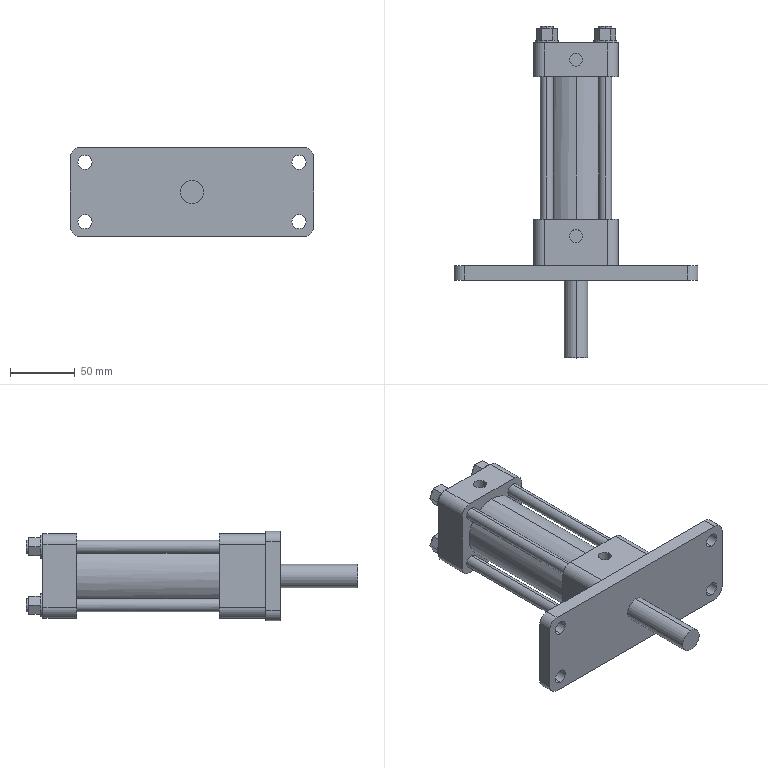Part | Creo | 1 solid | 108 faces | box 188 x 256 x 69 mm | volume 665930 mm3 | plane 56 | cylinder 52 | commonest cylinder face diameters 10 x20 16 x12 18 x10 11 x8 50 x2